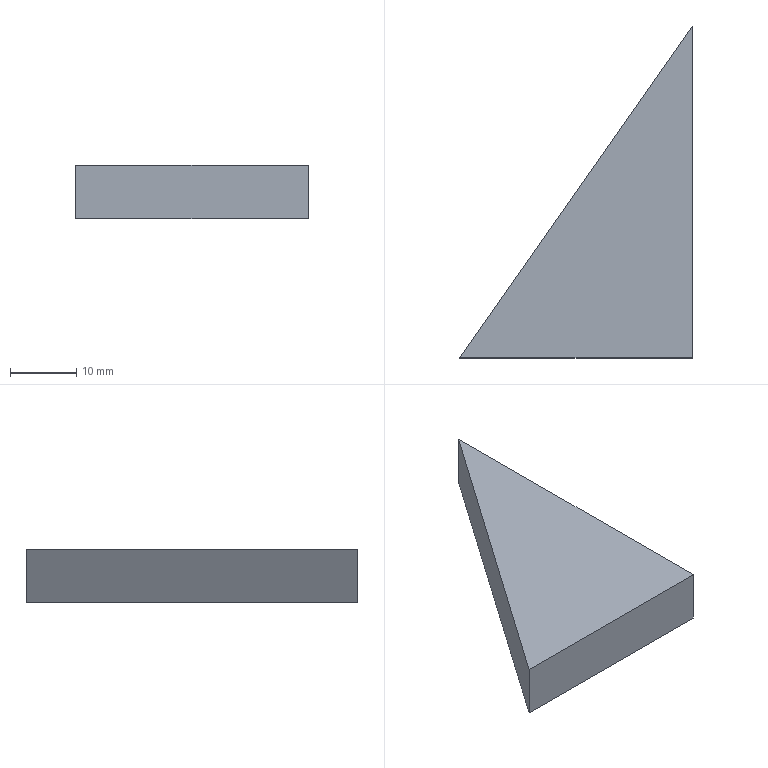Part | SolidWorks | features Extrusion 1 | 1 solid | 5 faces | box 35 x 50 x 8 mm | volume 7000 mm3 | plane 5
STEP:
#1=CARTESIAN_POINT('',(35.,50.,-4.));
#2=VERTEX_POINT('',#1);
#3=CARTESIAN_POINT('',(0.,0.,-4.));
#4=VERTEX_POINT('',#3);
#5=CARTESIAN_POINT('',(35.,50.,-4.));
#6=DIRECTION('',(-0.5735,-0.8192,0.));
#7=VECTOR('',#6,1000.);
#8=LINE('',#5,#7);
#9=EDGE_CURVE('',#2,#4,#8,.T.);
#10=ORIENTED_EDGE('',*,*,#9,.T.);
#11=CARTESIAN_POINT('',(0.,0.,4.));
#12=VERTEX_POINT('',#11);
#13=CARTESIAN_POINT('',(0.,0.,4.));
#14=DIRECTION('',(0.,0.,-1.));
#15=VECTOR('',#14,1000.);
#16=LINE('',#13,#15);
#17=EDGE_CURVE('',#12,#4,#16,.T.);
#18=ORIENTED_EDGE('',*,*,#17,.F.);
#19=CARTESIAN_POINT('',(35.,50.,4.));
#20=VERTEX_POINT('',#19);
#21=CARTESIAN_POINT('',(35.,50.,4.));
#22=DIRECTION('',(-0.5735,-0.8192,0.));
#23=VECTOR('',#22,1000.);
#24=LINE('',#21,#23);
#25=EDGE_CURVE('',#20,#12,#24,.T.);
#26=ORIENTED_EDGE('',*,*,#25,.F.);
#27=CARTESIAN_POINT('',(35.,50.,4.));
#28=DIRECTION('',(0.,0.,-1.));
#29=VECTOR('',#28,1000.);
#30=LINE('',#27,#29);
#31=EDGE_CURVE('',#20,#2,#30,.T.);
#32=ORIENTED_EDGE('',*,*,#31,.T.);
#33=EDGE_LOOP('',(#10,#18,#26,#32));
#34=FACE_OUTER_BOUND('',#33,.T.);
#35=CARTESIAN_POINT('',(35.,50.,4.));
#36=DIRECTION('',(0.8192,-0.5735,0.));
#37=DIRECTION('',(0.5735,0.8192,0.));
#38=AXIS2_PLACEMENT_3D('',#35,#36,#37);
#39=PLANE('',#38);
#40=ADVANCED_FACE('',(#34),#39,.F.);
#41=CARTESIAN_POINT('',(35.,0.,-4.));
#42=VERTEX_POINT('',#41);
#43=CARTESIAN_POINT('',(0.,0.,-4.));
#44=DIRECTION('',(1.,0.,0.));
#45=VECTOR('',#44,1000.);
#46=LINE('',#43,#45);
#47=EDGE_CURVE('',#4,#42,#46,.T.);
#48=ORIENTED_EDGE('',*,*,#47,.T.);
#49=CARTESIAN_POINT('',(35.,0.,4.));
#50=VERTEX_POINT('',#49);
#51=CARTESIAN_POINT('',(35.,0.,4.));
#52=DIRECTION('',(0.,0.,-1.));
#53=VECTOR('',#52,1000.);
#54=LINE('',#51,#53);
#55=EDGE_CURVE('',#50,#42,#54,.T.);
#56=ORIENTED_EDGE('',*,*,#55,.F.);
#57=CARTESIAN_POINT('',(0.,0.,4.));
#58=DIRECTION('',(1.,0.,0.));
#59=VECTOR('',#58,1000.);
#60=LINE('',#57,#59);
#61=EDGE_CURVE('',#12,#50,#60,.T.);
#62=ORIENTED_EDGE('',*,*,#61,.F.);
#63=ORIENTED_EDGE('',*,*,#17,.T.);
#64=EDGE_LOOP('',(#48,#56,#62,#63));
#65=FACE_OUTER_BOUND('',#64,.T.);
#66=CARTESIAN_POINT('',(0.,0.,4.));
#67=DIRECTION('',(0.,1.,0.));
#68=DIRECTION('',(0.,0.,1.));
#69=AXIS2_PLACEMENT_3D('',#66,#67,#68);
#70=PLANE('',#69);
#71=ADVANCED_FACE('',(#65),#70,.F.);
#72=CARTESIAN_POINT('',(35.,0.,-4.));
#73=DIRECTION('',(0.,1.,0.));
#74=VECTOR('',#73,1000.);
#75=LINE('',#72,#74);
#76=EDGE_CURVE('',#42,#2,#75,.T.);
#77=ORIENTED_EDGE('',*,*,#76,.T.);
#78=ORIENTED_EDGE('',*,*,#31,.F.);
#79=CARTESIAN_POINT('',(35.,0.,4.));
#80=DIRECTION('',(0.,1.,0.));
#81=VECTOR('',#80,1000.);
#82=LINE('',#79,#81);
#83=EDGE_CURVE('',#50,#20,#82,.T.);
#84=ORIENTED_EDGE('',*,*,#83,.F.);
#85=ORIENTED_EDGE('',*,*,#55,.T.);
#86=EDGE_LOOP('',(#77,#78,#84,#85));
#87=FACE_OUTER_BOUND('',#86,.T.);
#88=CARTESIAN_POINT('',(35.,0.,4.));
#89=DIRECTION('',(-1.,0.,0.));
#90=DIRECTION('',(0.,0.,1.));
#91=AXIS2_PLACEMENT_3D('',#88,#89,#90);
#92=PLANE('',#91);
#93=ADVANCED_FACE('',(#87),#92,.F.);
#94=ORIENTED_EDGE('',*,*,#25,.T.);
#95=ORIENTED_EDGE('',*,*,#61,.T.);
#96=ORIENTED_EDGE('',*,*,#83,.T.);
#97=EDGE_LOOP('',(#94,#95,#96));
#98=FACE_OUTER_BOUND('',#97,.T.);
#99=CARTESIAN_POINT('',(0.,0.,4.));
#100=DIRECTION('',(0.,0.,1.));
#101=DIRECTION('',(1.,0.,0.));
#102=AXIS2_PLACEMENT_3D('',#99,#100,#101);
#103=PLANE('',#102);
#104=ADVANCED_FACE('',(#98),#103,.T.);
#105=ORIENTED_EDGE('',*,*,#9,.F.);
#106=ORIENTED_EDGE('',*,*,#76,.F.);
#107=ORIENTED_EDGE('',*,*,#47,.F.);
#108=EDGE_LOOP('',(#105,#106,#107));
#109=FACE_OUTER_BOUND('',#108,.T.);
#110=CARTESIAN_POINT('',(0.,0.,-4.));
#111=DIRECTION('',(0.,0.,1.));
#112=DIRECTION('',(1.,0.,0.));
#113=AXIS2_PLACEMENT_3D('',#110,#111,#112);
#114=PLANE('',#113);
#115=ADVANCED_FACE('',(#109),#114,.F.);
#116=CLOSED_SHELL('',(#40,#71,#93,#104,#115));
#117=MANIFOLD_SOLID_BREP('',#116);
#118=CARTESIAN_POINT('',(0.,0.,0.));
#119=DIRECTION('',(0.,0.,1.));
#120=DIRECTION('',(1.,0.,0.));
#121=AXIS2_PLACEMENT_3D('',#118,#119,#120);
#122=(LENGTH_UNIT()NAMED_UNIT(*)SI_UNIT(.MILLI.,.METRE.));
#123=UNCERTAINTY_MEASURE_WITH_UNIT(LENGTH_MEASURE(0.00001),#122,'','');
#124=(NAMED_UNIT(*)PLANE_ANGLE_UNIT()SI_UNIT($,.RADIAN.));
#125=(NAMED_UNIT(*)SI_UNIT($,.STERADIAN.)SOLID_ANGLE_UNIT());
#126=(GEOMETRIC_REPRESENTATION_CONTEXT(3)GLOBAL_UNCERTAINTY_ASSIGNED_CONTEXT((#123))GLOBAL_UNIT_ASSIGNED_CONTEXT((#122,#124,#125))REPRESENTATION_CONTEXT('',''));
#127=ADVANCED_BREP_SHAPE_REPRESENTATION('',(#117,#121),#126);